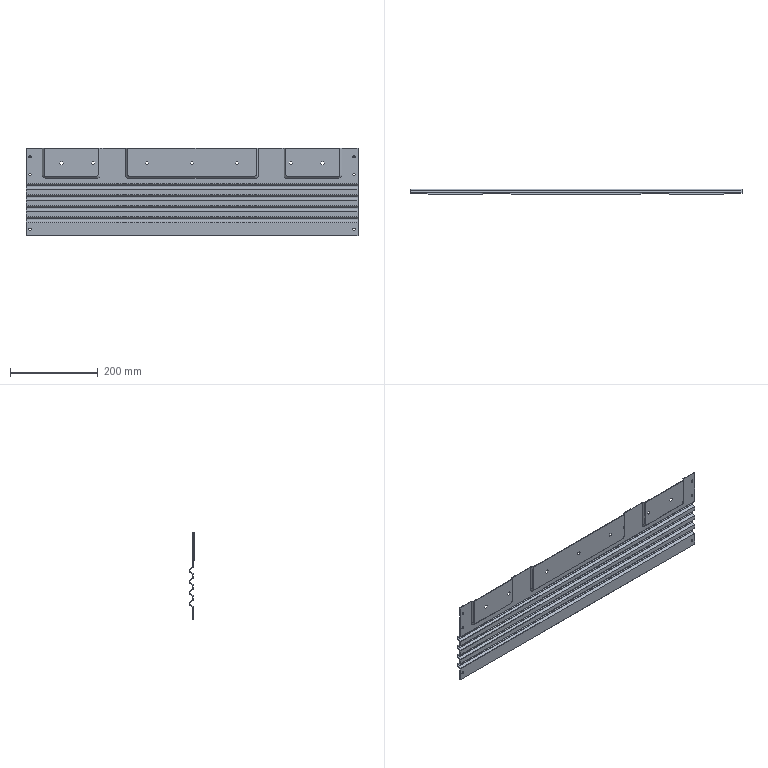Part | NX | features BREP 1 | 1 solid | 128 faces | box 755.2 x 13.6 x 200 mm | volume 214320 mm3 | plane 96 | cylinder 28 | cone 4 | commonest cylinder face diameters 5.1 x12 7.6 x4 10 x4 16.8 x4 17.6 x4